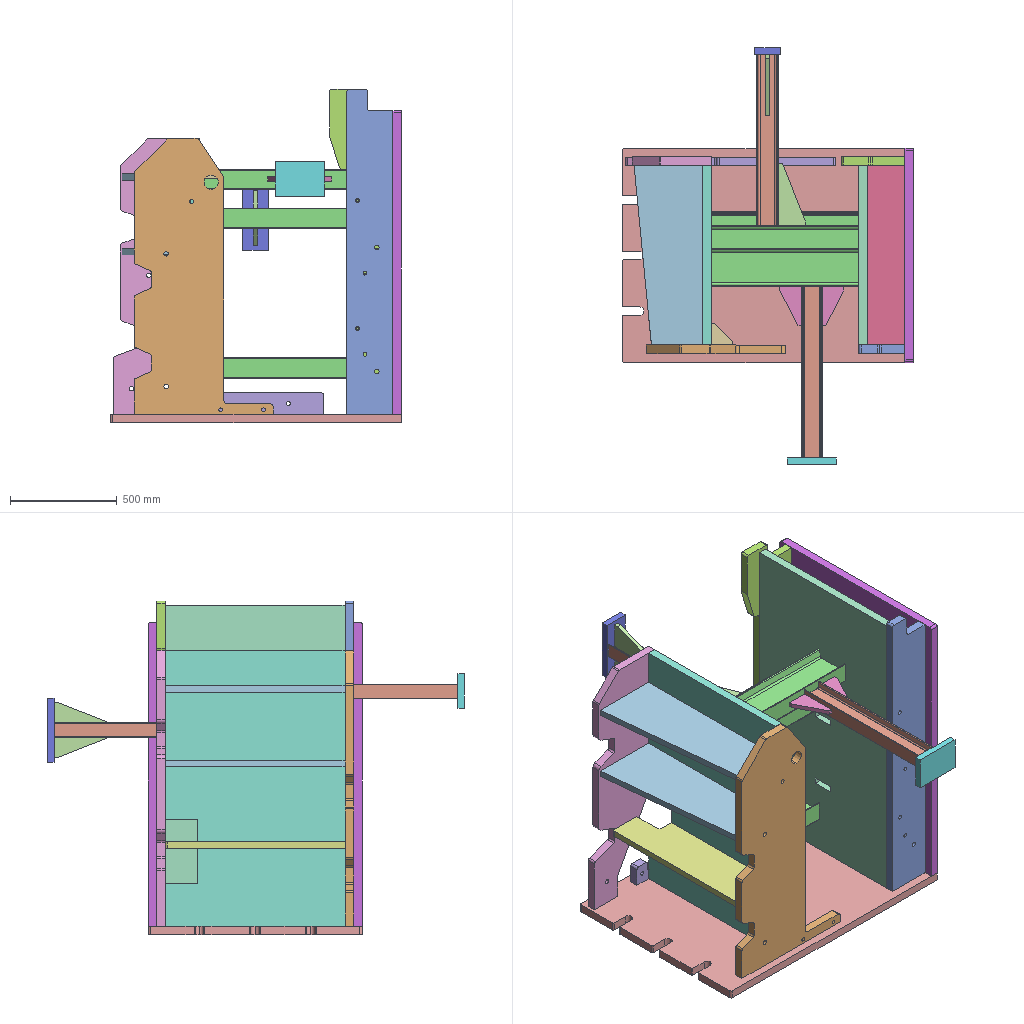Assembly | SolidWorks | 18 different items | 26 placed | box 1360 x 1948 x 1560 mm
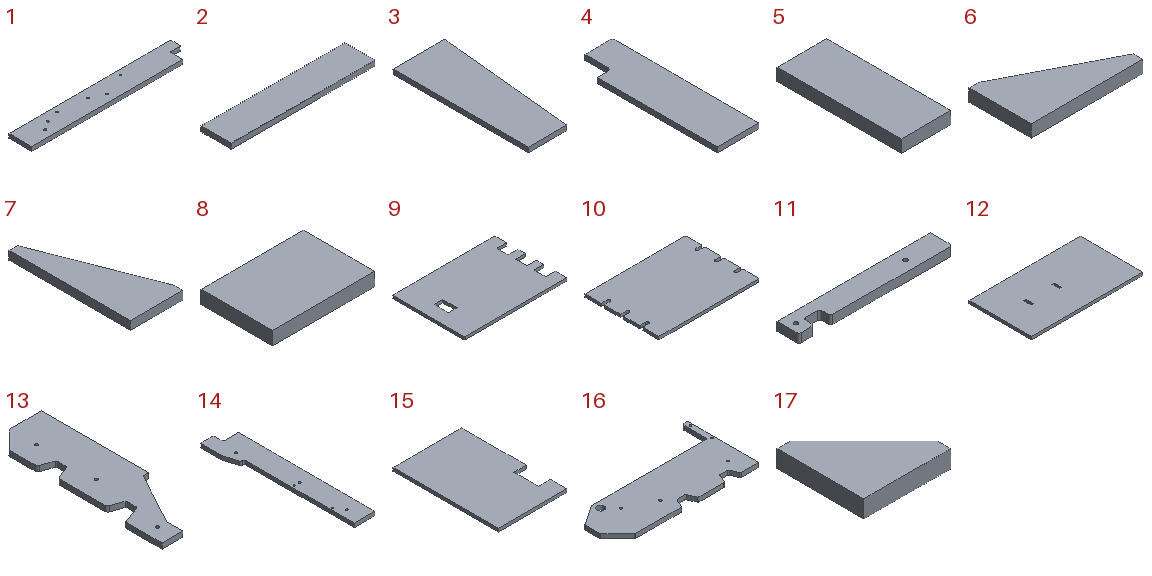Parts list (item | name | quantity | size | volume | features):
1 | - | x1 | 1520 x 215 x 40 mm | 12529786 mm3 | features 3DProfileFeature 2, HoleWzd 2, Extrusion 1, Fillet 1, ICE 1
2 | - | x3 | 840 x 175 x 30 mm | 4410000 mm3 | features Extrusion 1
3 | - | x2 | 320 x 840 x 30 mm | 7043400 mm3 | features Extrusion 1
4 | - | x1 | 239 x 840 x 30 mm | 5664731 mm3 | features Extrusion 1, Fillet 1
5 | - | x1 | 120 x 300 x 30 mm | 1080000 mm3 | features Extrusion 1
6 | - | x2 | 180 x 100 x 20 mm | 219750 mm3 | features Extrusion 1
7 | - | x3 | 125 x 289 x 20 mm | 440050 mm3 | features Extrusion 1
8 | - | x1 | 230 x 160 x 30 mm | 1104000 mm3 | features Extrusion 1
9 | - | x1 | 1420 x 1000 x 40 mm | 53251434 mm3 | features Extrusion 1, Fillet 1
10 | - | x1 | 1360 x 1000 x 40 mm | 53476912 mm3 | features Fillet 2, Extrusion 1
11 | - | x1 | 700 x 100 x 40 mm | 2627926 mm3 | features Extrusion 1, Fillet 1
12 | - | x1 | 1500 x 840 x 40 mm | 50160000 mm3 | features Extrusion 1
13 | - | x1 | 399 x 1290 x 40 mm | 14647498 mm3 | features Fillet 3, ICE 2, 3DProfileFeature 1, Chamfer 1, Extrusion 1, HoleWzd 1
14 | - | x1 | 295.68 x 1520 x 40 mm | 13433677 mm3 | features Fillet 2, 3DProfileFeature 1, Extrusion 1, HoleWzd 1
15 | - | x1 | 840 x 1290 x 40 mm | 41544000 mm3 | features Extrusion 1
16 | - | x1 | 1290 x 650 x 40 mm | 20252849 mm3 | features Fillet 3, Chamfer 2, 3DProfileFeature 1, Extrusion 1, HoleWzd 1, ICE 1
17 | - | x3 | 100 x 100 x 20 mm | 127750 mm3 | features Extrusion 1
18 | hot-rolled double t steel gb | x1 | - | - | -
Mates (type | each side: item.copy, entity, surface, feature):
Coincident | 10.1 face plane Boss-Extrude1 | 1.1 face plane Boss-Extrude1
DistanceDim | 10.1 face plane Boss-Extrude1 | 1.1 face plane Boss-Extrude1
DistanceDim | 1.1 face plane Boss-Extrude1 | 10.1 face plane Boss-Extrude1
Coincident | 10.1 face plane Boss-Extrude1 | 14.1 face plane Boss-Extrude1
Coincident | 14.1 face plane Boss-Extrude1 | 13.1 face plane Boss-Extrude1
Coincident | 10.1 face plane Boss-Extrude1 | 13.1 face plane Boss-Extrude1
DistanceDim | 14.1 face plane Boss-Extrude1 | 13.1 face plane Boss-Extrude1
Coincident | 10.1 face plane Boss-Extrude1 | 15.1 face plane Boss-Extrude1
Coincident | 13.1 face plane Boss-Extrude1 | 15.1 face plane Boss-Extrude1 | 2 times
Coincident | 10.1 face plane Boss-Extrude1 | 16.1 face plane Boss-Extrude1
Coincident | 1.1 face plane Boss-Extrude1 | 16.1 face plane Boss-Extrude1
Coincident | 10.1 face plane Boss-Extrude1 | 11.1 face plane Boss-Extrude1
Coincident | 13.1 face plane Boss-Extrude1 | 11.1 face plane Boss-Extrude1
Tangent | assembly face | 16.1 face cylinder Boss-Extrude1
Tangent | assembly face | 1.1 face cylinder Boss-Extrude1 | 2 times
DistanceDim | assembly face | 1.1 face plane Boss-Extrude1
Coincident | 1.1 face plane Boss-Extrude1 | 2.1 face plane Boss-Extrude1 | 2 times
Coincident | 14.1 face plane Boss-Extrude1 | 2.2 face plane Boss-Extrude1
DistanceDim | 2.2 face plane Boss-Extrude1 | 2.1 face plane Boss-Extrude1
Coincident | 14.1 face plane Boss-Extrude1 | 2.3 face plane Boss-Extrude1
Coincident | 15.1 face plane Boss-Extrude1 | 3.1 face plane Boss-Extrude1
Coincident | 16.1 face plane Boss-Extrude1 | 3.1 face plane Boss-Extrude1
Coincident | 2.2 face plane Boss-Extrude1 | 3.2 face plane Boss-Extrude1
Coincident | 16.1 face plane Boss-Extrude1 | 3.2 face plane Boss-Extrude1
Coincident | 15.1 face plane Boss-Extrude1 | 3.2 face plane Boss-Extrude1
Coincident | 16.1 face plane Boss-Extrude1 | 4.1 face plane Boss-Extrude1
Coincident | 15.1 face plane Boss-Extrude1 | 4.1 face plane Boss-Extrude1
Coincident | 10.1 face plane Boss-Extrude1 | 9.1 face plane Boss-Extrude1 | 3 times
Coincident | 2.3 face plane Boss-Extrude1 | 9.1 face plane Boss-Extrude1
Tangent | assembly face | 14.1 face cylinder Boss-Extrude1
Tangent | assembly face | 11.1 face cylinder Boss-Extrude1 | 2 times
DistanceDim | assembly face | 13.1 face plane Boss-Extrude1
Coincident | 1.1 face plane Boss-Extrude1 | 2.3 face plane Boss-Extrude1
Coincident | 14.1 face plane Boss-Extrude1 | 9.1 face plane Boss-Extrude1
DistanceDim | 4.1 face plane Boss-Extrude1 | 10.1 face plane Boss-Extrude1
Coincident | 1.1 face plane Boss-Extrude1 | 2.2 face plane Boss-Extrude1
Coincident | 10.1 face plane Boss-Extrude1 | 12.1 face plane Boss-Extrude1
Coincident | 14.1 face plane Boss-Extrude1 | 12.1 face plane Boss-Extrude1 | 2 times
Coincident | 2.1 face plane Boss-Extrude1 | 4.1 face plane Boss-Extrude1
Coincident | 2.3 face plane Boss-Extrude1 | 3.1 face plane Boss-Extrude1
DistanceDim | 5.1 face plane Boss-Extrude1 | 7.1 face plane Boss-Extrude1
Coincident | 5.1 face plane Boss-Extrude1 | 7.2 face plane Boss-Extrude1
Coincident | 5.1 face plane Boss-Extrude1 | 7.3 face plane Boss-Extrude1
Coincident | 7.2 face plane Boss-Extrude1 | 7.3 face plane Boss-Extrude1
Coincident | 16.1 face plane Boss-Extrude1 | assembly face
Tangent | 16.1 face cylinder Boss-Extrude1 | assembly face
Parallel | 10.1 face plane Boss-Extrude1 | assembly face
DistanceDim | 16.1 face plane Boss-Extrude1 | 10.1 face plane Boss-Extrude1
DistanceDim | assembly face | 12.1 face plane Boss-Extrude1
Coincident | 6.1 face plane Boss-Extrude1 | 6.2 face plane Boss-Extrude1 | 2 times
DistanceDim | 11.1 face plane Boss-Extrude1 | 9.1 face plane Boss-Extrude1
Coincident | 17.1 face plane Boss-Extrude1 | 17.2 face plane Boss-Extrude1 | 2 times
Coincident | 17.3 face plane Boss-Extrude1 | 17.1 face plane Boss-Extrude1 | 2 times
Coincident | 4.1 face plane Boss-Extrude1 | 17.2 face plane Boss-Extrude1
Coincident | 3.2 face plane Boss-Extrude1 | 17.1 face plane Boss-Extrude1
Coincident | 3.1 face plane Boss-Extrude1 | 17.3 face plane Boss-Extrude1
Coincident | 16.1 face plane Boss-Extrude1 | 17.3 face plane Boss-Extrude1
Coincident | 15.1 face plane Boss-Extrude1 | 17.3 face plane Boss-Extrude1